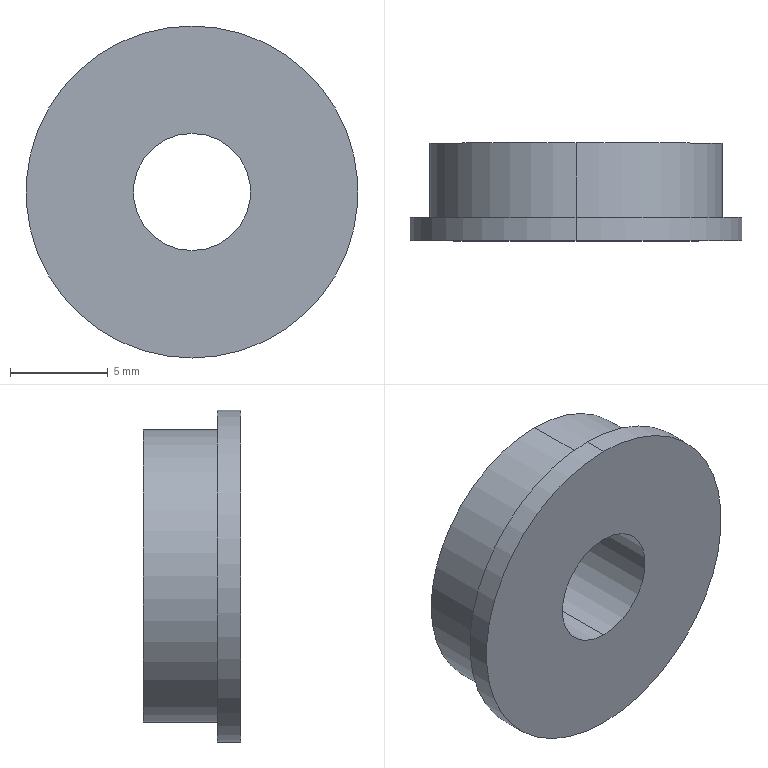Part | SolidWorks | features Revolution 1 | 1 solid | 9 faces | box 17 x 5 x 17 mm | volume 802.52 mm3 | cylinder 6 | plane 3 | commonest cylinder face diameters 6 x2 15 x2 17 x2
STEP:
#1=CARTESIAN_POINT('',(0.,4.599,-7.5));
#2=VERTEX_POINT('',#1);
#3=CARTESIAN_POINT('',(0.,4.599,7.5));
#4=VERTEX_POINT('',#3);
#5=CARTESIAN_POINT('',(0.,4.599,0.));
#6=DIRECTION('',(0.,-1.,0.));
#7=DIRECTION('',(0.,0.,-1.));
#8=AXIS2_PLACEMENT_3D('',#5,#6,#7);
#9=CIRCLE('',#8,7.5);
#10=EDGE_CURVE('',#2,#4,#9,.T.);
#11=ORIENTED_EDGE('',*,*,#10,.T.);
#12=CARTESIAN_POINT('',(0.,0.7991,7.5));
#13=VERTEX_POINT('',#12);
#14=CARTESIAN_POINT('',(0.,0.,7.5));
#15=DIRECTION('',(0.,-1.,0.));
#16=VECTOR('',#15,1000.);
#17=LINE('',#14,#16);
#18=EDGE_CURVE('',#4,#13,#17,.T.);
#19=ORIENTED_EDGE('',*,*,#18,.T.);
#20=CARTESIAN_POINT('',(0.,0.7991,-7.5));
#21=VERTEX_POINT('',#20);
#22=CARTESIAN_POINT('',(0.,0.7991,0.));
#23=DIRECTION('',(0.,-1.,0.));
#24=DIRECTION('',(0.,0.,-1.));
#25=AXIS2_PLACEMENT_3D('',#22,#23,#24);
#26=CIRCLE('',#25,7.5);
#27=EDGE_CURVE('',#21,#13,#26,.T.);
#28=ORIENTED_EDGE('',*,*,#27,.F.);
#29=CARTESIAN_POINT('',(0.,0.,-7.5));
#30=DIRECTION('',(0.,-1.,0.));
#31=VECTOR('',#30,1000.);
#32=LINE('',#29,#31);
#33=EDGE_CURVE('',#2,#21,#32,.T.);
#34=ORIENTED_EDGE('',*,*,#33,.F.);
#35=EDGE_LOOP('',(#11,#19,#28,#34));
#36=FACE_OUTER_BOUND('',#35,.T.);
#37=CARTESIAN_POINT('',(0.,0.,0.));
#38=DIRECTION('',(0.,-1.,0.));
#39=DIRECTION('',(0.,0.,-1.));
#40=AXIS2_PLACEMENT_3D('',#37,#38,#39);
#41=CYLINDRICAL_SURFACE('',#40,7.5);
#42=ADVANCED_FACE('',(#36),#41,.T.);
#43=CARTESIAN_POINT('',(0.,0.7991,-8.5));
#44=VERTEX_POINT('',#43);
#45=CARTESIAN_POINT('',(0.,0.7991,8.5));
#46=VERTEX_POINT('',#45);
#47=CARTESIAN_POINT('',(0.,0.7991,0.));
#48=DIRECTION('',(0.,-1.,0.));
#49=DIRECTION('',(0.,0.,-1.));
#50=AXIS2_PLACEMENT_3D('',#47,#48,#49);
#51=CIRCLE('',#50,8.5);
#52=EDGE_CURVE('',#44,#46,#51,.T.);
#53=ORIENTED_EDGE('',*,*,#52,.T.);
#54=CARTESIAN_POINT('',(0.,-0.4009,8.5));
#55=VERTEX_POINT('',#54);
#56=CARTESIAN_POINT('',(0.,0.,8.5));
#57=DIRECTION('',(0.,-1.,0.));
#58=VECTOR('',#57,1000.);
#59=LINE('',#56,#58);
#60=EDGE_CURVE('',#46,#55,#59,.T.);
#61=ORIENTED_EDGE('',*,*,#60,.T.);
#62=CARTESIAN_POINT('',(0.,-0.4009,-8.5));
#63=VERTEX_POINT('',#62);
#64=CARTESIAN_POINT('',(0.,-0.4009,0.));
#65=DIRECTION('',(0.,-1.,0.));
#66=DIRECTION('',(0.,0.,-1.));
#67=AXIS2_PLACEMENT_3D('',#64,#65,#66);
#68=CIRCLE('',#67,8.5);
#69=EDGE_CURVE('',#63,#55,#68,.T.);
#70=ORIENTED_EDGE('',*,*,#69,.F.);
#71=CARTESIAN_POINT('',(0.,0.,-8.5));
#72=DIRECTION('',(0.,-1.,0.));
#73=VECTOR('',#72,1000.);
#74=LINE('',#71,#73);
#75=EDGE_CURVE('',#44,#63,#74,.T.);
#76=ORIENTED_EDGE('',*,*,#75,.F.);
#77=EDGE_LOOP('',(#53,#61,#70,#76));
#78=FACE_OUTER_BOUND('',#77,.T.);
#79=CARTESIAN_POINT('',(0.,0.,0.));
#80=DIRECTION('',(0.,-1.,0.));
#81=DIRECTION('',(0.,0.,-1.));
#82=AXIS2_PLACEMENT_3D('',#79,#80,#81);
#83=CYLINDRICAL_SURFACE('',#82,8.5);
#84=ADVANCED_FACE('',(#78),#83,.T.);
#85=CARTESIAN_POINT('',(0.,4.599,3.));
#86=VERTEX_POINT('',#85);
#87=CARTESIAN_POINT('',(0.,4.599,-3.));
#88=VERTEX_POINT('',#87);
#89=CARTESIAN_POINT('',(0.,4.599,0.));
#90=DIRECTION('',(0.,-1.,0.));
#91=DIRECTION('',(0.,0.,-1.));
#92=AXIS2_PLACEMENT_3D('',#89,#90,#91);
#93=CIRCLE('',#92,3.);
#94=EDGE_CURVE('',#86,#88,#93,.T.);
#95=ORIENTED_EDGE('',*,*,#94,.F.);
#96=CARTESIAN_POINT('',(0.,-0.4009,3.));
#97=VERTEX_POINT('',#96);
#98=CARTESIAN_POINT('',(0.,0.,3.));
#99=DIRECTION('',(0.,-1.,0.));
#100=VECTOR('',#99,1000.);
#101=LINE('',#98,#100);
#102=EDGE_CURVE('',#86,#97,#101,.T.);
#103=ORIENTED_EDGE('',*,*,#102,.T.);
#104=CARTESIAN_POINT('',(0.,-0.4009,-3.));
#105=VERTEX_POINT('',#104);
#106=CARTESIAN_POINT('',(0.,-0.4009,0.));
#107=DIRECTION('',(0.,-1.,0.));
#108=DIRECTION('',(0.,0.,-1.));
#109=AXIS2_PLACEMENT_3D('',#106,#107,#108);
#110=CIRCLE('',#109,3.);
#111=EDGE_CURVE('',#97,#105,#110,.T.);
#112=ORIENTED_EDGE('',*,*,#111,.T.);
#113=CARTESIAN_POINT('',(0.,0.,-3.));
#114=DIRECTION('',(0.,-1.,0.));
#115=VECTOR('',#114,1000.);
#116=LINE('',#113,#115);
#117=EDGE_CURVE('',#88,#105,#116,.T.);
#118=ORIENTED_EDGE('',*,*,#117,.F.);
#119=EDGE_LOOP('',(#95,#103,#112,#118));
#120=FACE_OUTER_BOUND('',#119,.T.);
#121=CARTESIAN_POINT('',(0.,0.,0.));
#122=DIRECTION('',(0.,-1.,0.));
#123=DIRECTION('',(0.,0.,-1.));
#124=AXIS2_PLACEMENT_3D('',#121,#122,#123);
#125=CYLINDRICAL_SURFACE('',#124,3.);
#126=ADVANCED_FACE('',(#120),#125,.F.);
#127=CARTESIAN_POINT('',(0.,4.599,0.));
#128=DIRECTION('',(0.,-1.,0.));
#129=DIRECTION('',(0.,0.,-1.));
#130=AXIS2_PLACEMENT_3D('',#127,#128,#129);
#131=CIRCLE('',#130,3.);
#132=EDGE_CURVE('',#88,#86,#131,.T.);
#133=ORIENTED_EDGE('',*,*,#132,.T.);
#134=ORIENTED_EDGE('',*,*,#94,.T.);
#135=EDGE_LOOP('',(#133,#134));
#136=FACE_BOUND('',#135,.T.);
#137=ORIENTED_EDGE('',*,*,#10,.F.);
#138=CARTESIAN_POINT('',(0.,4.599,0.));
#139=DIRECTION('',(0.,-1.,0.));
#140=DIRECTION('',(0.,0.,-1.));
#141=AXIS2_PLACEMENT_3D('',#138,#139,#140);
#142=CIRCLE('',#141,7.5);
#143=EDGE_CURVE('',#4,#2,#142,.T.);
#144=ORIENTED_EDGE('',*,*,#143,.F.);
#145=EDGE_LOOP('',(#137,#144));
#146=FACE_OUTER_BOUND('',#145,.T.);
#147=CARTESIAN_POINT('',(7.5,4.599,0.));
#148=DIRECTION('',(0.,1.,0.));
#149=DIRECTION('',(0.,0.,1.));
#150=AXIS2_PLACEMENT_3D('',#147,#148,#149);
#151=PLANE('',#150);
#152=ADVANCED_FACE('',(#136,#146),#151,.T.);
#153=ORIENTED_EDGE('',*,*,#102,.F.);
#154=ORIENTED_EDGE('',*,*,#132,.F.);
#155=ORIENTED_EDGE('',*,*,#117,.T.);
#156=CARTESIAN_POINT('',(0.,-0.4009,0.));
#157=DIRECTION('',(0.,-1.,0.));
#158=DIRECTION('',(0.,0.,-1.));
#159=AXIS2_PLACEMENT_3D('',#156,#157,#158);
#160=CIRCLE('',#159,3.);
#161=EDGE_CURVE('',#105,#97,#160,.T.);
#162=ORIENTED_EDGE('',*,*,#161,.T.);
#163=EDGE_LOOP('',(#153,#154,#155,#162));
#164=FACE_OUTER_BOUND('',#163,.T.);
#165=CARTESIAN_POINT('',(0.,0.,0.));
#166=DIRECTION('',(0.,-1.,0.));
#167=DIRECTION('',(0.,0.,-1.));
#168=AXIS2_PLACEMENT_3D('',#165,#166,#167);
#169=CYLINDRICAL_SURFACE('',#168,3.);
#170=ADVANCED_FACE('',(#164),#169,.F.);
#171=ORIENTED_EDGE('',*,*,#69,.T.);
#172=CARTESIAN_POINT('',(0.,-0.4009,0.));
#173=DIRECTION('',(0.,-1.,0.));
#174=DIRECTION('',(0.,0.,-1.));
#175=AXIS2_PLACEMENT_3D('',#172,#173,#174);
#176=CIRCLE('',#175,8.5);
#177=EDGE_CURVE('',#55,#63,#176,.T.);
#178=ORIENTED_EDGE('',*,*,#177,.T.);
#179=EDGE_LOOP('',(#171,#178));
#180=FACE_OUTER_BOUND('',#179,.T.);
#181=ORIENTED_EDGE('',*,*,#161,.F.);
#182=ORIENTED_EDGE('',*,*,#111,.F.);
#183=EDGE_LOOP('',(#181,#182));
#184=FACE_BOUND('',#183,.T.);
#185=CARTESIAN_POINT('',(3.,-0.4009,0.));
#186=DIRECTION('',(0.,-1.,0.));
#187=DIRECTION('',(0.,0.,-1.));
#188=AXIS2_PLACEMENT_3D('',#185,#186,#187);
#189=PLANE('',#188);
#190=ADVANCED_FACE('',(#180,#184),#189,.T.);
#191=ORIENTED_EDGE('',*,*,#60,.F.);
#192=CARTESIAN_POINT('',(0.,0.7991,0.));
#193=DIRECTION('',(0.,-1.,0.));
#194=DIRECTION('',(0.,0.,-1.));
#195=AXIS2_PLACEMENT_3D('',#192,#193,#194);
#196=CIRCLE('',#195,8.5);
#197=EDGE_CURVE('',#46,#44,#196,.T.);
#198=ORIENTED_EDGE('',*,*,#197,.T.);
#199=ORIENTED_EDGE('',*,*,#75,.T.);
#200=ORIENTED_EDGE('',*,*,#177,.F.);
#201=EDGE_LOOP('',(#191,#198,#199,#200));
#202=FACE_OUTER_BOUND('',#201,.T.);
#203=CARTESIAN_POINT('',(0.,0.,0.));
#204=DIRECTION('',(0.,-1.,0.));
#205=DIRECTION('',(0.,0.,-1.));
#206=AXIS2_PLACEMENT_3D('',#203,#204,#205);
#207=CYLINDRICAL_SURFACE('',#206,8.5);
#208=ADVANCED_FACE('',(#202),#207,.T.);
#209=ORIENTED_EDGE('',*,*,#27,.T.);
#210=CARTESIAN_POINT('',(0.,0.7991,0.));
#211=DIRECTION('',(0.,-1.,0.));
#212=DIRECTION('',(0.,0.,-1.));
#213=AXIS2_PLACEMENT_3D('',#210,#211,#212);
#214=CIRCLE('',#213,7.5);
#215=EDGE_CURVE('',#13,#21,#214,.T.);
#216=ORIENTED_EDGE('',*,*,#215,.T.);
#217=EDGE_LOOP('',(#209,#216));
#218=FACE_BOUND('',#217,.T.);
#219=ORIENTED_EDGE('',*,*,#52,.F.);
#220=ORIENTED_EDGE('',*,*,#197,.F.);
#221=EDGE_LOOP('',(#219,#220));
#222=FACE_OUTER_BOUND('',#221,.T.);
#223=CARTESIAN_POINT('',(8.5,0.7991,0.));
#224=DIRECTION('',(0.,1.,0.));
#225=DIRECTION('',(0.,0.,1.));
#226=AXIS2_PLACEMENT_3D('',#223,#224,#225);
#227=PLANE('',#226);
#228=ADVANCED_FACE('',(#218,#222),#227,.T.);
#229=ORIENTED_EDGE('',*,*,#18,.F.);
#230=ORIENTED_EDGE('',*,*,#143,.T.);
#231=ORIENTED_EDGE('',*,*,#33,.T.);
#232=ORIENTED_EDGE('',*,*,#215,.F.);
#233=EDGE_LOOP('',(#229,#230,#231,#232));
#234=FACE_OUTER_BOUND('',#233,.T.);
#235=CARTESIAN_POINT('',(0.,0.,0.));
#236=DIRECTION('',(0.,-1.,0.));
#237=DIRECTION('',(0.,0.,-1.));
#238=AXIS2_PLACEMENT_3D('',#235,#236,#237);
#239=CYLINDRICAL_SURFACE('',#238,7.5);
#240=ADVANCED_FACE('',(#234),#239,.T.);
#241=CLOSED_SHELL('',(#42,#84,#126,#152,#170,#190,#208,#228,#240));
#242=MANIFOLD_SOLID_BREP('',#241);
#243=CARTESIAN_POINT('',(0.,0.,0.));
#244=DIRECTION('',(0.,0.,1.));
#245=DIRECTION('',(1.,0.,0.));
#246=AXIS2_PLACEMENT_3D('',#243,#244,#245);
#247=(LENGTH_UNIT()NAMED_UNIT(*)SI_UNIT(.MILLI.,.METRE.));
#248=UNCERTAINTY_MEASURE_WITH_UNIT(LENGTH_MEASURE(0.00001),#247,'','');
#249=(NAMED_UNIT(*)PLANE_ANGLE_UNIT()SI_UNIT($,.RADIAN.));
#250=(NAMED_UNIT(*)SI_UNIT($,.STERADIAN.)SOLID_ANGLE_UNIT());
#251=(GEOMETRIC_REPRESENTATION_CONTEXT(3)GLOBAL_UNCERTAINTY_ASSIGNED_CONTEXT((#248))GLOBAL_UNIT_ASSIGNED_CONTEXT((#247,#249,#250))REPRESENTATION_CONTEXT('',''));
#252=ADVANCED_BREP_SHAPE_REPRESENTATION('',(#242,#246),#251);